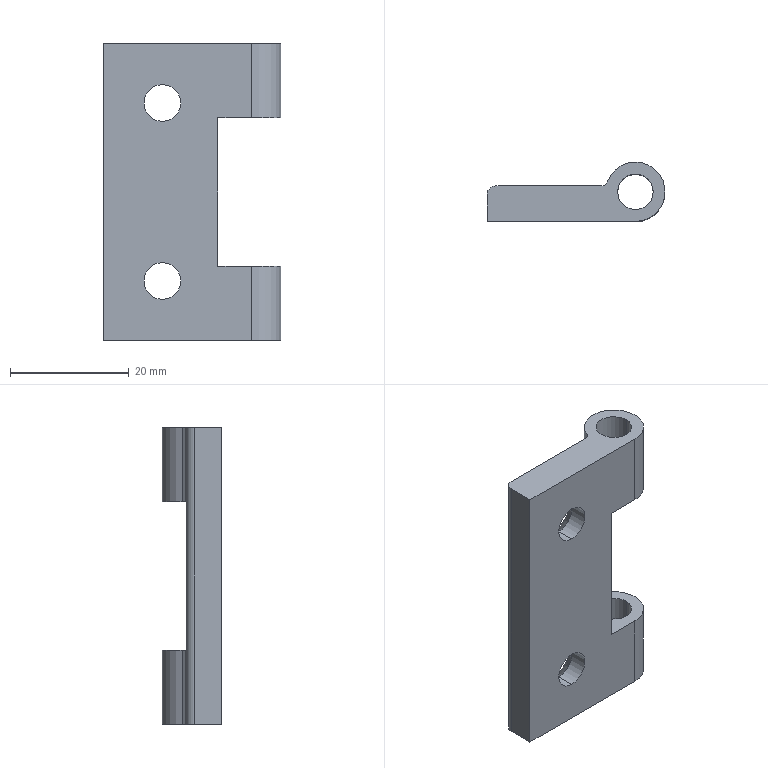Part | STEP file | 750038561 | 1 solid | 25 faces | box 30 x 10 x 50 mm | volume 6694 mm3 | cylinder 13 | plane 8 | cone 4 | commonest cylinder face diameters 6 x4 6.2 x4 2 x2 10 x2 3 x1
STEP:
#1=CARTESIAN_POINT('',(-15.,0.,18.1));
#2=VERTEX_POINT('',#1);
#3=CARTESIAN_POINT('',(-15.,0.,11.9));
#4=VERTEX_POINT('',#3);
#5=CARTESIAN_POINT('',(-15.,0.,15.));
#6=DIRECTION('',(0.,-1.,0.));
#7=DIRECTION('',(0.,0.,1.));
#8=AXIS2_PLACEMENT_3D('',#5,#6,#7);
#9=CIRCLE('',#8,3.1);
#10=EDGE_CURVE('',#2,#4,#9,.T.);
#11=ORIENTED_EDGE('',*,*,#10,.T.);
#12=CARTESIAN_POINT('',(-15.,3.1,11.9));
#13=VERTEX_POINT('',#12);
#14=CARTESIAN_POINT('',(-15.,-54994.,11.9));
#15=DIRECTION('',(0.,1.,0.));
#16=VECTOR('',#15,1000.);
#17=LINE('',#14,#16);
#18=EDGE_CURVE('',#4,#13,#17,.T.);
#19=ORIENTED_EDGE('',*,*,#18,.T.);
#20=CARTESIAN_POINT('',(-15.,3.1,18.1));
#21=VERTEX_POINT('',#20);
#22=CARTESIAN_POINT('',(-15.,3.1,15.));
#23=DIRECTION('',(0.,-1.,0.));
#24=DIRECTION('',(0.,0.,1.));
#25=AXIS2_PLACEMENT_3D('',#22,#23,#24);
#26=CIRCLE('',#25,3.1);
#27=EDGE_CURVE('',#21,#13,#26,.T.);
#28=ORIENTED_EDGE('',*,*,#27,.F.);
#29=CARTESIAN_POINT('',(-15.,-54994.,18.1));
#30=DIRECTION('',(0.,1.,0.));
#31=VECTOR('',#30,1000.);
#32=LINE('',#29,#31);
#33=EDGE_CURVE('',#2,#21,#32,.T.);
#34=ORIENTED_EDGE('',*,*,#33,.F.);
#35=EDGE_LOOP('',(#11,#19,#28,#34));
#36=FACE_OUTER_BOUND('',#35,.T.);
#37=CARTESIAN_POINT('',(-15.,-54994.,15.));
#38=DIRECTION('',(0.,1.,0.));
#39=DIRECTION('',(0.,0.,1.));
#40=AXIS2_PLACEMENT_3D('',#37,#38,#39);
#41=CYLINDRICAL_SURFACE('',#40,3.1);
#42=ADVANCED_FACE('',(#36),#41,.F.);
#43=CARTESIAN_POINT('',(-15.,0.,-11.9));
#44=VERTEX_POINT('',#43);
#45=CARTESIAN_POINT('',(-15.,0.,-18.1));
#46=VERTEX_POINT('',#45);
#47=CARTESIAN_POINT('',(-15.,0.,-15.));
#48=DIRECTION('',(0.,-1.,0.));
#49=DIRECTION('',(0.,0.,1.));
#50=AXIS2_PLACEMENT_3D('',#47,#48,#49);
#51=CIRCLE('',#50,3.1);
#52=EDGE_CURVE('',#44,#46,#51,.T.);
#53=ORIENTED_EDGE('',*,*,#52,.T.);
#54=CARTESIAN_POINT('',(-15.,3.1,-18.1));
#55=VERTEX_POINT('',#54);
#56=CARTESIAN_POINT('',(-15.,-54994.,-18.1));
#57=DIRECTION('',(0.,1.,0.));
#58=VECTOR('',#57,1000.);
#59=LINE('',#56,#58);
#60=EDGE_CURVE('',#46,#55,#59,.T.);
#61=ORIENTED_EDGE('',*,*,#60,.T.);
#62=CARTESIAN_POINT('',(-15.,3.1,-11.9));
#63=VERTEX_POINT('',#62);
#64=CARTESIAN_POINT('',(-15.,3.1,-15.));
#65=DIRECTION('',(0.,-1.,0.));
#66=DIRECTION('',(0.,0.,1.));
#67=AXIS2_PLACEMENT_3D('',#64,#65,#66);
#68=CIRCLE('',#67,3.1);
#69=EDGE_CURVE('',#63,#55,#68,.T.);
#70=ORIENTED_EDGE('',*,*,#69,.F.);
#71=CARTESIAN_POINT('',(-15.,-54994.,-11.9));
#72=DIRECTION('',(0.,1.,0.));
#73=VECTOR('',#72,1000.);
#74=LINE('',#71,#73);
#75=EDGE_CURVE('',#44,#63,#74,.T.);
#76=ORIENTED_EDGE('',*,*,#75,.F.);
#77=EDGE_LOOP('',(#53,#61,#70,#76));
#78=FACE_OUTER_BOUND('',#77,.T.);
#79=CARTESIAN_POINT('',(-15.,-54994.,-15.));
#80=DIRECTION('',(0.,1.,0.));
#81=DIRECTION('',(0.,0.,1.));
#82=AXIS2_PLACEMENT_3D('',#79,#80,#81);
#83=CYLINDRICAL_SURFACE('',#82,3.1);
#84=ADVANCED_FACE('',(#78),#83,.F.);
#85=CARTESIAN_POINT('',(3.,5.,25.));
#86=VERTEX_POINT('',#85);
#87=CARTESIAN_POINT('',(-3.,5.,25.));
#88=VERTEX_POINT('',#87);
#89=CARTESIAN_POINT('',(0.,5.,25.));
#90=DIRECTION('',(0.,0.,-1.));
#91=DIRECTION('',(-1.,0.,0.));
#92=AXIS2_PLACEMENT_3D('',#89,#90,#91);
#93=CIRCLE('',#92,3.);
#94=EDGE_CURVE('',#86,#88,#93,.T.);
#95=ORIENTED_EDGE('',*,*,#94,.F.);
#96=CARTESIAN_POINT('',(3.,5.,12.5));
#97=VERTEX_POINT('',#96);
#98=CARTESIAN_POINT('',(3.,5.,25.));
#99=DIRECTION('',(0.,0.,-1.));
#100=VECTOR('',#99,1000.);
#101=LINE('',#98,#100);
#102=EDGE_CURVE('',#86,#97,#101,.T.);
#103=ORIENTED_EDGE('',*,*,#102,.T.);
#104=CARTESIAN_POINT('',(-3.,5.,12.5));
#105=VERTEX_POINT('',#104);
#106=CARTESIAN_POINT('',(0.,5.,12.5));
#107=DIRECTION('',(0.,0.,1.));
#108=DIRECTION('',(-1.,0.,0.));
#109=AXIS2_PLACEMENT_3D('',#106,#107,#108);
#110=CIRCLE('',#109,3.);
#111=EDGE_CURVE('',#105,#97,#110,.T.);
#112=ORIENTED_EDGE('',*,*,#111,.F.);
#113=CARTESIAN_POINT('',(-3.,5.,25.));
#114=DIRECTION('',(0.,0.,-1.));
#115=VECTOR('',#114,1000.);
#116=LINE('',#113,#115);
#117=EDGE_CURVE('',#88,#105,#116,.T.);
#118=ORIENTED_EDGE('',*,*,#117,.F.);
#119=EDGE_LOOP('',(#95,#103,#112,#118));
#120=FACE_OUTER_BOUND('',#119,.T.);
#121=CARTESIAN_POINT('',(0.,5.,25.));
#122=DIRECTION('',(0.,0.,-1.));
#123=DIRECTION('',(-1.,0.,0.));
#124=AXIS2_PLACEMENT_3D('',#121,#122,#123);
#125=CYLINDRICAL_SURFACE('',#124,3.);
#126=ADVANCED_FACE('',(#120),#125,.F.);
#127=CARTESIAN_POINT('',(3.,5.,-12.5));
#128=VERTEX_POINT('',#127);
#129=CARTESIAN_POINT('',(-3.,5.,-12.5));
#130=VERTEX_POINT('',#129);
#131=CARTESIAN_POINT('',(0.,5.,-12.5));
#132=DIRECTION('',(0.,0.,-1.));
#133=DIRECTION('',(-1.,0.,0.));
#134=AXIS2_PLACEMENT_3D('',#131,#132,#133);
#135=CIRCLE('',#134,3.);
#136=EDGE_CURVE('',#128,#130,#135,.T.);
#137=ORIENTED_EDGE('',*,*,#136,.F.);
#138=CARTESIAN_POINT('',(3.,5.,-25.));
#139=VERTEX_POINT('',#138);
#140=CARTESIAN_POINT('',(3.,5.,25.));
#141=DIRECTION('',(0.,0.,-1.));
#142=VECTOR('',#141,1000.);
#143=LINE('',#140,#142);
#144=EDGE_CURVE('',#128,#139,#143,.T.);
#145=ORIENTED_EDGE('',*,*,#144,.T.);
#146=CARTESIAN_POINT('',(-3.,5.,-25.));
#147=VERTEX_POINT('',#146);
#148=CARTESIAN_POINT('',(0.,5.,-25.));
#149=DIRECTION('',(0.,0.,-1.));
#150=DIRECTION('',(-1.,0.,0.));
#151=AXIS2_PLACEMENT_3D('',#148,#149,#150);
#152=CIRCLE('',#151,3.);
#153=EDGE_CURVE('',#139,#147,#152,.T.);
#154=ORIENTED_EDGE('',*,*,#153,.T.);
#155=CARTESIAN_POINT('',(-3.,5.,25.));
#156=DIRECTION('',(0.,0.,-1.));
#157=VECTOR('',#156,1000.);
#158=LINE('',#155,#157);
#159=EDGE_CURVE('',#130,#147,#158,.T.);
#160=ORIENTED_EDGE('',*,*,#159,.F.);
#161=EDGE_LOOP('',(#137,#145,#154,#160));
#162=FACE_OUTER_BOUND('',#161,.T.);
#163=CARTESIAN_POINT('',(0.,5.,25.));
#164=DIRECTION('',(0.,0.,-1.));
#165=DIRECTION('',(-1.,0.,0.));
#166=AXIS2_PLACEMENT_3D('',#163,#164,#165);
#167=CYLINDRICAL_SURFACE('',#166,3.);
#168=ADVANCED_FACE('',(#162),#167,.F.);
#169=ORIENTED_EDGE('',*,*,#27,.T.);
#170=CARTESIAN_POINT('',(-15.,6.,9.));
#171=VERTEX_POINT('',#170);
#172=CARTESIAN_POINT('',(-15.,6.,9.));
#173=DIRECTION('',(0.,0.7071,-0.7071));
#174=VECTOR('',#173,1000.);
#175=LINE('',#172,#174);
#176=EDGE_CURVE('',#13,#171,#175,.T.);
#177=ORIENTED_EDGE('',*,*,#176,.T.);
#178=CARTESIAN_POINT('',(-15.,6.,21.));
#179=VERTEX_POINT('',#178);
#180=CARTESIAN_POINT('',(-15.,6.,15.));
#181=DIRECTION('',(0.,1.,0.));
#182=DIRECTION('',(0.,0.,1.));
#183=AXIS2_PLACEMENT_3D('',#180,#181,#182);
#184=CIRCLE('',#183,6.);
#185=EDGE_CURVE('',#171,#179,#184,.T.);
#186=ORIENTED_EDGE('',*,*,#185,.T.);
#187=CARTESIAN_POINT('',(-15.,6.,21.));
#188=DIRECTION('',(0.,0.7071,0.7071));
#189=VECTOR('',#188,1000.);
#190=LINE('',#187,#189);
#191=EDGE_CURVE('',#21,#179,#190,.T.);
#192=ORIENTED_EDGE('',*,*,#191,.F.);
#193=EDGE_LOOP('',(#169,#177,#186,#192));
#194=FACE_OUTER_BOUND('',#193,.T.);
#195=CARTESIAN_POINT('',(-15.,6.,15.));
#196=DIRECTION('',(0.,1.,0.));
#197=DIRECTION('',(0.,0.,1.));
#198=AXIS2_PLACEMENT_3D('',#195,#196,#197);
#199=CONICAL_SURFACE('',#198,6.,0.7854);
#200=ADVANCED_FACE('',(#194),#199,.F.);
#201=ORIENTED_EDGE('',*,*,#69,.T.);
#202=CARTESIAN_POINT('',(-15.,6.,-21.));
#203=VERTEX_POINT('',#202);
#204=CARTESIAN_POINT('',(-15.,6.,-21.));
#205=DIRECTION('',(0.,0.7071,-0.7071));
#206=VECTOR('',#205,1000.);
#207=LINE('',#204,#206);
#208=EDGE_CURVE('',#55,#203,#207,.T.);
#209=ORIENTED_EDGE('',*,*,#208,.T.);
#210=CARTESIAN_POINT('',(-15.,6.,-9.));
#211=VERTEX_POINT('',#210);
#212=CARTESIAN_POINT('',(-15.,6.,-15.));
#213=DIRECTION('',(0.,1.,0.));
#214=DIRECTION('',(0.,0.,1.));
#215=AXIS2_PLACEMENT_3D('',#212,#213,#214);
#216=CIRCLE('',#215,6.);
#217=EDGE_CURVE('',#203,#211,#216,.T.);
#218=ORIENTED_EDGE('',*,*,#217,.T.);
#219=CARTESIAN_POINT('',(-15.,6.,-9.));
#220=DIRECTION('',(0.,0.7071,0.7071));
#221=VECTOR('',#220,1000.);
#222=LINE('',#219,#221);
#223=EDGE_CURVE('',#63,#211,#222,.T.);
#224=ORIENTED_EDGE('',*,*,#223,.F.);
#225=EDGE_LOOP('',(#201,#209,#218,#224));
#226=FACE_OUTER_BOUND('',#225,.T.);
#227=CARTESIAN_POINT('',(-15.,6.,-15.));
#228=DIRECTION('',(0.,1.,0.));
#229=DIRECTION('',(0.,0.,1.));
#230=AXIS2_PLACEMENT_3D('',#227,#228,#229);
#231=CONICAL_SURFACE('',#230,6.,0.7854);
#232=ADVANCED_FACE('',(#226),#231,.F.);
#233=CARTESIAN_POINT('',(0.,0.,25.));
#234=VERTEX_POINT('',#233);
#235=CARTESIAN_POINT('',(0.,0.,12.5));
#236=VERTEX_POINT('',#235);
#237=CARTESIAN_POINT('',(0.,0.,25.));
#238=DIRECTION('',(0.,0.,-1.));
#239=VECTOR('',#238,1000.);
#240=LINE('',#237,#239);
#241=EDGE_CURVE('',#234,#236,#240,.T.);
#242=ORIENTED_EDGE('',*,*,#241,.F.);
#243=CARTESIAN_POINT('',(-25.,0.,25.));
#244=VERTEX_POINT('',#243);
#245=CARTESIAN_POINT('',(-25.,0.,25.));
#246=DIRECTION('',(1.,0.,0.));
#247=VECTOR('',#246,1000.);
#248=LINE('',#245,#247);
#249=EDGE_CURVE('',#244,#234,#248,.T.);
#250=ORIENTED_EDGE('',*,*,#249,.F.);
#251=CARTESIAN_POINT('',(-25.,0.,-25.));
#252=VERTEX_POINT('',#251);
#253=CARTESIAN_POINT('',(-25.,0.,25.));
#254=DIRECTION('',(0.,0.,1.));
#255=VECTOR('',#254,1000.);
#256=LINE('',#253,#255);
#257=EDGE_CURVE('',#252,#244,#256,.T.);
#258=ORIENTED_EDGE('',*,*,#257,.F.);
#259=CARTESIAN_POINT('',(0.,0.,-25.));
#260=VERTEX_POINT('',#259);
#261=CARTESIAN_POINT('',(-25.,0.,-25.));
#262=DIRECTION('',(-1.,0.,0.));
#263=VECTOR('',#262,1000.);
#264=LINE('',#261,#263);
#265=EDGE_CURVE('',#260,#252,#264,.T.);
#266=ORIENTED_EDGE('',*,*,#265,.F.);
#267=CARTESIAN_POINT('',(0.,0.,-12.5));
#268=VERTEX_POINT('',#267);
#269=CARTESIAN_POINT('',(0.,0.,25.));
#270=DIRECTION('',(0.,0.,-1.));
#271=VECTOR('',#270,1000.);
#272=LINE('',#269,#271);
#273=EDGE_CURVE('',#268,#260,#272,.T.);
#274=ORIENTED_EDGE('',*,*,#273,.F.);
#275=CARTESIAN_POINT('',(-5.657,0.,-12.5));
#276=VERTEX_POINT('',#275);
#277=CARTESIAN_POINT('',(-25.,0.,-12.5));
#278=DIRECTION('',(1.,0.,0.));
#279=VECTOR('',#278,1000.);
#280=LINE('',#277,#279);
#281=EDGE_CURVE('',#276,#268,#280,.T.);
#282=ORIENTED_EDGE('',*,*,#281,.F.);
#283=CARTESIAN_POINT('',(-5.657,0.,12.5));
#284=VERTEX_POINT('',#283);
#285=CARTESIAN_POINT('',(-5.657,0.,25.));
#286=DIRECTION('',(0.,0.,-1.));
#287=VECTOR('',#286,1000.);
#288=LINE('',#285,#287);
#289=EDGE_CURVE('',#284,#276,#288,.T.);
#290=ORIENTED_EDGE('',*,*,#289,.F.);
#291=CARTESIAN_POINT('',(-25.,0.,12.5));
#292=DIRECTION('',(-1.,0.,0.));
#293=VECTOR('',#292,1000.);
#294=LINE('',#291,#293);
#295=EDGE_CURVE('',#236,#284,#294,.T.);
#296=ORIENTED_EDGE('',*,*,#295,.F.);
#297=EDGE_LOOP('',(#242,#250,#258,#266,#274,#282,#290,#296));
#298=FACE_OUTER_BOUND('',#297,.T.);
#299=ORIENTED_EDGE('',*,*,#10,.F.);
#300=CARTESIAN_POINT('',(-15.,0.,15.));
#301=DIRECTION('',(0.,-1.,0.));
#302=DIRECTION('',(0.,0.,1.));
#303=AXIS2_PLACEMENT_3D('',#300,#301,#302);
#304=CIRCLE('',#303,3.1);
#305=EDGE_CURVE('',#4,#2,#304,.T.);
#306=ORIENTED_EDGE('',*,*,#305,.F.);
#307=EDGE_LOOP('',(#299,#306));
#308=FACE_BOUND('',#307,.T.);
#309=ORIENTED_EDGE('',*,*,#52,.F.);
#310=CARTESIAN_POINT('',(-15.,0.,-15.));
#311=DIRECTION('',(0.,-1.,0.));
#312=DIRECTION('',(0.,0.,1.));
#313=AXIS2_PLACEMENT_3D('',#310,#311,#312);
#314=CIRCLE('',#313,3.1);
#315=EDGE_CURVE('',#46,#44,#314,.T.);
#316=ORIENTED_EDGE('',*,*,#315,.F.);
#317=EDGE_LOOP('',(#309,#316));
#318=FACE_BOUND('',#317,.T.);
#319=CARTESIAN_POINT('',(-25.,0.,25.));
#320=DIRECTION('',(0.,1.,0.));
#321=DIRECTION('',(-1.,0.,0.));
#322=AXIS2_PLACEMENT_3D('',#319,#320,#321);
#323=PLANE('',#322);
#324=ADVANCED_FACE('',(#298,#308,#318),#323,.F.);
#325=CARTESIAN_POINT('',(-5.657,6.,12.5));
#326=VERTEX_POINT('',#325);
#327=CARTESIAN_POINT('',(-4.714,6.667,12.5));
#328=VERTEX_POINT('',#327);
#329=CARTESIAN_POINT('',(-5.657,7.,12.5));
#330=DIRECTION('',(0.,0.,1.));
#331=DIRECTION('',(-1.,0.,0.));
#332=AXIS2_PLACEMENT_3D('',#329,#330,#331);
#333=CIRCLE('',#332,1.);
#334=EDGE_CURVE('',#326,#328,#333,.T.);
#335=ORIENTED_EDGE('',*,*,#334,.T.);
#336=CARTESIAN_POINT('',(0.,5.,12.5));
#337=DIRECTION('',(0.,0.,-1.));
#338=DIRECTION('',(-1.,0.,0.));
#339=AXIS2_PLACEMENT_3D('',#336,#337,#338);
#340=CIRCLE('',#339,5.);
#341=EDGE_CURVE('',#328,#236,#340,.T.);
#342=ORIENTED_EDGE('',*,*,#341,.T.);
#343=ORIENTED_EDGE('',*,*,#295,.T.);
#344=CARTESIAN_POINT('',(-5.657,31.,12.5));
#345=DIRECTION('',(0.,1.,0.));
#346=VECTOR('',#345,1000.);
#347=LINE('',#344,#346);
#348=EDGE_CURVE('',#284,#326,#347,.T.);
#349=ORIENTED_EDGE('',*,*,#348,.T.);
#350=EDGE_LOOP('',(#335,#342,#343,#349));
#351=FACE_OUTER_BOUND('',#350,.T.);
#352=ORIENTED_EDGE('',*,*,#111,.T.);
#353=CARTESIAN_POINT('',(0.,5.,12.5));
#354=DIRECTION('',(0.,0.,1.));
#355=DIRECTION('',(-1.,0.,0.));
#356=AXIS2_PLACEMENT_3D('',#353,#354,#355);
#357=CIRCLE('',#356,3.);
#358=EDGE_CURVE('',#97,#105,#357,.T.);
#359=ORIENTED_EDGE('',*,*,#358,.T.);
#360=EDGE_LOOP('',(#352,#359));
#361=FACE_BOUND('',#360,.T.);
#362=CARTESIAN_POINT('',(-5.657,31.,12.5));
#363=DIRECTION('',(0.,0.,-1.));
#364=DIRECTION('',(-1.,0.,0.));
#365=AXIS2_PLACEMENT_3D('',#362,#363,#364);
#366=PLANE('',#365);
#367=ADVANCED_FACE('',(#351,#361),#366,.T.);
#368=CARTESIAN_POINT('',(-4.714,6.667,25.));
#369=VERTEX_POINT('',#368);
#370=CARTESIAN_POINT('',(0.,5.,25.));
#371=DIRECTION('',(0.,0.,-1.));
#372=DIRECTION('',(-1.,0.,0.));
#373=AXIS2_PLACEMENT_3D('',#370,#371,#372);
#374=CIRCLE('',#373,5.);
#375=EDGE_CURVE('',#369,#234,#374,.T.);
#376=ORIENTED_EDGE('',*,*,#375,.T.);
#377=ORIENTED_EDGE('',*,*,#241,.T.);
#378=ORIENTED_EDGE('',*,*,#341,.F.);
#379=CARTESIAN_POINT('',(-4.714,6.667,25.));
#380=DIRECTION('',(0.,0.,1.));
#381=VECTOR('',#380,1000.);
#382=LINE('',#379,#381);
#383=EDGE_CURVE('',#328,#369,#382,.T.);
#384=ORIENTED_EDGE('',*,*,#383,.T.);
#385=EDGE_LOOP('',(#376,#377,#378,#384));
#386=FACE_OUTER_BOUND('',#385,.T.);
#387=CARTESIAN_POINT('',(0.,5.,25.));
#388=DIRECTION('',(0.,0.,-1.));
#389=DIRECTION('',(-1.,0.,0.));
#390=AXIS2_PLACEMENT_3D('',#387,#388,#389);
#391=CYLINDRICAL_SURFACE('',#390,5.);
#392=ADVANCED_FACE('',(#386),#391,.T.);
#393=CARTESIAN_POINT('',(0.,5.,25.));
#394=DIRECTION('',(0.,0.,-1.));
#395=DIRECTION('',(-1.,0.,0.));
#396=AXIS2_PLACEMENT_3D('',#393,#394,#395);
#397=CIRCLE('',#396,3.);
#398=EDGE_CURVE('',#88,#86,#397,.T.);
#399=ORIENTED_EDGE('',*,*,#398,.T.);
#400=ORIENTED_EDGE('',*,*,#94,.T.);
#401=EDGE_LOOP('',(#399,#400));
#402=FACE_BOUND('',#401,.T.);
#403=CARTESIAN_POINT('',(-5.657,6.,25.));
#404=VERTEX_POINT('',#403);
#405=CARTESIAN_POINT('',(-23.5,6.,25.));
#406=VERTEX_POINT('',#405);
#407=CARTESIAN_POINT('',(0.,6.,25.));
#408=DIRECTION('',(-1.,0.,0.));
#409=VECTOR('',#408,1000.);
#410=LINE('',#407,#409);
#411=EDGE_CURVE('',#404,#406,#410,.T.);
#412=ORIENTED_EDGE('',*,*,#411,.T.);
#413=CARTESIAN_POINT('',(-25.,4.5,25.));
#414=VERTEX_POINT('',#413);
#415=CARTESIAN_POINT('',(-23.5,4.5,25.));
#416=DIRECTION('',(0.,0.,1.));
#417=DIRECTION('',(-1.,0.,0.));
#418=AXIS2_PLACEMENT_3D('',#415,#416,#417);
#419=CIRCLE('',#418,1.5);
#420=EDGE_CURVE('',#406,#414,#419,.T.);
#421=ORIENTED_EDGE('',*,*,#420,.T.);
#422=CARTESIAN_POINT('',(-25.,5.,25.));
#423=DIRECTION('',(0.,-1.,0.));
#424=VECTOR('',#423,1000.);
#425=LINE('',#422,#424);
#426=EDGE_CURVE('',#414,#244,#425,.T.);
#427=ORIENTED_EDGE('',*,*,#426,.T.);
#428=ORIENTED_EDGE('',*,*,#249,.T.);
#429=ORIENTED_EDGE('',*,*,#375,.F.);
#430=CARTESIAN_POINT('',(-5.657,7.,25.));
#431=DIRECTION('',(0.,0.,-1.));
#432=DIRECTION('',(-1.,0.,0.));
#433=AXIS2_PLACEMENT_3D('',#430,#431,#432);
#434=CIRCLE('',#433,1.);
#435=EDGE_CURVE('',#369,#404,#434,.T.);
#436=ORIENTED_EDGE('',*,*,#435,.T.);
#437=EDGE_LOOP('',(#412,#421,#427,#428,#429,#436));
#438=FACE_OUTER_BOUND('',#437,.T.);
#439=CARTESIAN_POINT('',(0.,5.,25.));
#440=DIRECTION('',(0.,0.,1.));
#441=DIRECTION('',(1.,0.,0.));
#442=AXIS2_PLACEMENT_3D('',#439,#440,#441);
#443=PLANE('',#442);
#444=ADVANCED_FACE('',(#402,#438),#443,.T.);
#445=ORIENTED_EDGE('',*,*,#257,.T.);
#446=ORIENTED_EDGE('',*,*,#426,.F.);
#447=CARTESIAN_POINT('',(-25.,4.5,-25.));
#448=VERTEX_POINT('',#447);
#449=CARTESIAN_POINT('',(-25.,4.5,25.));
#450=DIRECTION('',(0.,0.,1.));
#451=VECTOR('',#450,1000.);
#452=LINE('',#449,#451);
#453=EDGE_CURVE('',#448,#414,#452,.T.);
#454=ORIENTED_EDGE('',*,*,#453,.F.);
#455=CARTESIAN_POINT('',(-25.,4.5,-25.));
#456=DIRECTION('',(0.,1.,0.));
#457=VECTOR('',#456,1000.);
#458=LINE('',#455,#457);
#459=EDGE_CURVE('',#252,#448,#458,.T.);
#460=ORIENTED_EDGE('',*,*,#459,.F.);
#461=EDGE_LOOP('',(#445,#446,#454,#460));
#462=FACE_OUTER_BOUND('',#461,.T.);
#463=CARTESIAN_POINT('',(-25.,4.5,25.));
#464=DIRECTION('',(1.,0.,0.));
#465=DIRECTION('',(0.,0.,-1.));
#466=AXIS2_PLACEMENT_3D('',#463,#464,#465);
#467=PLANE('',#466);
#468=ADVANCED_FACE('',(#462),#467,.F.);
#469=CARTESIAN_POINT('',(0.,5.,-25.));
#470=DIRECTION('',(0.,0.,-1.));
#471=DIRECTION('',(-1.,0.,0.));
#472=AXIS2_PLACEMENT_3D('',#469,#470,#471);
#473=CIRCLE('',#472,3.);
#474=EDGE_CURVE('',#147,#139,#473,.T.);
#475=ORIENTED_EDGE('',*,*,#474,.F.);
#476=ORIENTED_EDGE('',*,*,#153,.F.);
#477=EDGE_LOOP('',(#475,#476));
#478=FACE_BOUND('',#477,.T.);
#479=CARTESIAN_POINT('',(-23.5,6.,-25.));
#480=VERTEX_POINT('',#479);
#481=CARTESIAN_POINT('',(-23.5,4.5,-25.));
#482=DIRECTION('',(0.,0.,1.));
#483=DIRECTION('',(-1.,0.,0.));
#484=AXIS2_PLACEMENT_3D('',#481,#482,#483);
#485=CIRCLE('',#484,1.5);
#486=EDGE_CURVE('',#480,#448,#485,.T.);
#487=ORIENTED_EDGE('',*,*,#486,.F.);
#488=CARTESIAN_POINT('',(-5.657,6.,-25.));
#489=VERTEX_POINT('',#488);
#490=CARTESIAN_POINT('',(0.,6.,-25.));
#491=DIRECTION('',(-1.,0.,0.));
#492=VECTOR('',#491,1000.);
#493=LINE('',#490,#492);
#494=EDGE_CURVE('',#489,#480,#493,.T.);
#495=ORIENTED_EDGE('',*,*,#494,.F.);
#496=CARTESIAN_POINT('',(-4.714,6.667,-25.));
#497=VERTEX_POINT('',#496);
#498=CARTESIAN_POINT('',(-5.657,7.,-25.));
#499=DIRECTION('',(0.,0.,1.));
#500=DIRECTION('',(-1.,0.,0.));
#501=AXIS2_PLACEMENT_3D('',#498,#499,#500);
#502=CIRCLE('',#501,1.);
#503=EDGE_CURVE('',#489,#497,#502,.T.);
#504=ORIENTED_EDGE('',*,*,#503,.T.);
#505=CARTESIAN_POINT('',(0.,5.,-25.));
#506=DIRECTION('',(0.,0.,1.));
#507=DIRECTION('',(-1.,0.,0.));
#508=AXIS2_PLACEMENT_3D('',#505,#506,#507);
#509=CIRCLE('',#508,5.);
#510=EDGE_CURVE('',#260,#497,#509,.T.);
#511=ORIENTED_EDGE('',*,*,#510,.F.);
#512=ORIENTED_EDGE('',*,*,#265,.T.);
#513=ORIENTED_EDGE('',*,*,#459,.T.);
#514=EDGE_LOOP('',(#487,#495,#504,#511,#512,#513));
#515=FACE_OUTER_BOUND('',#514,.T.);
#516=CARTESIAN_POINT('',(0.,5.,-25.));
#517=DIRECTION('',(0.,0.,1.));
#518=DIRECTION('',(1.,0.,0.));
#519=AXIS2_PLACEMENT_3D('',#516,#517,#518);
#520=PLANE('',#519);
#521=ADVANCED_FACE('',(#478,#515),#520,.F.);
#522=ORIENTED_EDGE('',*,*,#273,.T.);
#523=ORIENTED_EDGE('',*,*,#510,.T.);
#524=CARTESIAN_POINT('',(-4.714,6.667,-12.5));
#525=VERTEX_POINT('',#524);
#526=CARTESIAN_POINT('',(-4.714,6.667,25.));
#527=DIRECTION('',(0.,0.,1.));
#528=VECTOR('',#527,1000.);
#529=LINE('',#526,#528);
#530=EDGE_CURVE('',#497,#525,#529,.T.);
#531=ORIENTED_EDGE('',*,*,#530,.T.);
#532=CARTESIAN_POINT('',(0.,5.,-12.5));
#533=DIRECTION('',(0.,0.,-1.));
#534=DIRECTION('',(-1.,0.,0.));
#535=AXIS2_PLACEMENT_3D('',#532,#533,#534);
#536=CIRCLE('',#535,5.);
#537=EDGE_CURVE('',#525,#268,#536,.T.);
#538=ORIENTED_EDGE('',*,*,#537,.T.);
#539=EDGE_LOOP('',(#522,#523,#531,#538));
#540=FACE_OUTER_BOUND('',#539,.T.);
#541=CARTESIAN_POINT('',(0.,5.,25.));
#542=DIRECTION('',(0.,0.,-1.));
#543=DIRECTION('',(-1.,0.,0.));
#544=AXIS2_PLACEMENT_3D('',#541,#542,#543);
#545=CYLINDRICAL_SURFACE('',#544,5.);
#546=ADVANCED_FACE('',(#540),#545,.T.);
#547=CARTESIAN_POINT('',(-5.657,6.,-12.5));
#548=VERTEX_POINT('',#547);
#549=CARTESIAN_POINT('',(-5.657,7.,-12.5));
#550=DIRECTION('',(0.,0.,-1.));
#551=DIRECTION('',(-1.,0.,0.));
#552=AXIS2_PLACEMENT_3D('',#549,#550,#551);
#553=CIRCLE('',#552,1.);
#554=EDGE_CURVE('',#525,#548,#553,.T.);
#555=ORIENTED_EDGE('',*,*,#554,.T.);
#556=CARTESIAN_POINT('',(-5.657,31.,-12.5));
#557=DIRECTION('',(0.,-1.,0.));
#558=VECTOR('',#557,1000.);
#559=LINE('',#556,#558);
#560=EDGE_CURVE('',#548,#276,#559,.T.);
#561=ORIENTED_EDGE('',*,*,#560,.T.);
#562=ORIENTED_EDGE('',*,*,#281,.T.);
#563=ORIENTED_EDGE('',*,*,#537,.F.);
#564=EDGE_LOOP('',(#555,#561,#562,#563));
#565=FACE_OUTER_BOUND('',#564,.T.);
#566=CARTESIAN_POINT('',(0.,5.,-12.5));
#567=DIRECTION('',(0.,0.,-1.));
#568=DIRECTION('',(-1.,0.,0.));
#569=AXIS2_PLACEMENT_3D('',#566,#567,#568);
#570=CIRCLE('',#569,3.);
#571=EDGE_CURVE('',#130,#128,#570,.T.);
#572=ORIENTED_EDGE('',*,*,#571,.T.);
#573=ORIENTED_EDGE('',*,*,#136,.T.);
#574=EDGE_LOOP('',(#572,#573));
#575=FACE_BOUND('',#574,.T.);
#576=CARTESIAN_POINT('',(5.,31.,-12.5));
#577=DIRECTION('',(0.,0.,1.));
#578=DIRECTION('',(1.,0.,0.));
#579=AXIS2_PLACEMENT_3D('',#576,#577,#578);
#580=PLANE('',#579);
#581=ADVANCED_FACE('',(#565,#575),#580,.T.);
#582=CARTESIAN_POINT('',(-5.657,6.,-12.5));
#583=DIRECTION('',(0.,0.,1.));
#584=VECTOR('',#583,1000.);
#585=LINE('',#582,#584);
#586=EDGE_CURVE('',#548,#326,#585,.T.);
#587=ORIENTED_EDGE('',*,*,#586,.T.);
#588=ORIENTED_EDGE('',*,*,#348,.F.);
#589=ORIENTED_EDGE('',*,*,#289,.T.);
#590=ORIENTED_EDGE('',*,*,#560,.F.);
#591=EDGE_LOOP('',(#587,#588,#589,#590));
#592=FACE_OUTER_BOUND('',#591,.T.);
#593=CARTESIAN_POINT('',(-5.657,31.,-12.5));
#594=DIRECTION('',(1.,0.,0.));
#595=DIRECTION('',(0.,0.,-1.));
#596=AXIS2_PLACEMENT_3D('',#593,#594,#595);
#597=PLANE('',#596);
#598=ADVANCED_FACE('',(#592),#597,.T.);
#599=ORIENTED_EDGE('',*,*,#18,.F.);
#600=ORIENTED_EDGE('',*,*,#305,.T.);
#601=ORIENTED_EDGE('',*,*,#33,.T.);
#602=CARTESIAN_POINT('',(-15.,3.1,15.));
#603=DIRECTION('',(0.,-1.,0.));
#604=DIRECTION('',(0.,0.,1.));
#605=AXIS2_PLACEMENT_3D('',#602,#603,#604);
#606=CIRCLE('',#605,3.1);
#607=EDGE_CURVE('',#13,#21,#606,.T.);
#608=ORIENTED_EDGE('',*,*,#607,.F.);
#609=EDGE_LOOP('',(#599,#600,#601,#608));
#610=FACE_OUTER_BOUND('',#609,.T.);
#611=CARTESIAN_POINT('',(-15.,-54994.,15.));
#612=DIRECTION('',(0.,1.,0.));
#613=DIRECTION('',(0.,0.,1.));
#614=AXIS2_PLACEMENT_3D('',#611,#612,#613);
#615=CYLINDRICAL_SURFACE('',#614,3.1);
#616=ADVANCED_FACE('',(#610),#615,.F.);
#617=ORIENTED_EDGE('',*,*,#60,.F.);
#618=ORIENTED_EDGE('',*,*,#315,.T.);
#619=ORIENTED_EDGE('',*,*,#75,.T.);
#620=CARTESIAN_POINT('',(-15.,3.1,-15.));
#621=DIRECTION('',(0.,-1.,0.));
#622=DIRECTION('',(0.,0.,1.));
#623=AXIS2_PLACEMENT_3D('',#620,#621,#622);
#624=CIRCLE('',#623,3.1);
#625=EDGE_CURVE('',#55,#63,#624,.T.);
#626=ORIENTED_EDGE('',*,*,#625,.F.);
#627=EDGE_LOOP('',(#617,#618,#619,#626));
#628=FACE_OUTER_BOUND('',#627,.T.);
#629=CARTESIAN_POINT('',(-15.,-54994.,-15.));
#630=DIRECTION('',(0.,1.,0.));
#631=DIRECTION('',(0.,0.,1.));
#632=AXIS2_PLACEMENT_3D('',#629,#630,#631);
#633=CYLINDRICAL_SURFACE('',#632,3.1);
#634=ADVANCED_FACE('',(#628),#633,.F.);
#635=ORIENTED_EDGE('',*,*,#102,.F.);
#636=ORIENTED_EDGE('',*,*,#398,.F.);
#637=ORIENTED_EDGE('',*,*,#117,.T.);
#638=ORIENTED_EDGE('',*,*,#358,.F.);
#639=EDGE_LOOP('',(#635,#636,#637,#638));
#640=FACE_OUTER_BOUND('',#639,.T.);
#641=CARTESIAN_POINT('',(0.,5.,25.));
#642=DIRECTION('',(0.,0.,-1.));
#643=DIRECTION('',(-1.,0.,0.));
#644=AXIS2_PLACEMENT_3D('',#641,#642,#643);
#645=CYLINDRICAL_SURFACE('',#644,3.);
#646=ADVANCED_FACE('',(#640),#645,.F.);
#647=CARTESIAN_POINT('',(-5.657,6.,25.));
#648=DIRECTION('',(0.,0.,-1.));
#649=VECTOR('',#648,1000.);
#650=LINE('',#647,#649);
#651=EDGE_CURVE('',#404,#326,#650,.T.);
#652=ORIENTED_EDGE('',*,*,#651,.F.);
#653=ORIENTED_EDGE('',*,*,#435,.F.);
#654=ORIENTED_EDGE('',*,*,#383,.F.);
#655=ORIENTED_EDGE('',*,*,#334,.F.);
#656=EDGE_LOOP('',(#652,#653,#654,#655));
#657=FACE_OUTER_BOUND('',#656,.T.);
#658=CARTESIAN_POINT('',(-5.657,7.,25.));
#659=DIRECTION('',(0.,0.,-1.));
#660=DIRECTION('',(-1.,0.,0.));
#661=AXIS2_PLACEMENT_3D('',#658,#659,#660);
#662=CYLINDRICAL_SURFACE('',#661,1.);
#663=ADVANCED_FACE('',(#657),#662,.F.);
#664=ORIENTED_EDGE('',*,*,#420,.F.);
#665=CARTESIAN_POINT('',(-23.5,6.,25.));
#666=DIRECTION('',(0.,0.,-1.));
#667=VECTOR('',#666,1000.);
#668=LINE('',#665,#667);
#669=EDGE_CURVE('',#406,#480,#668,.T.);
#670=ORIENTED_EDGE('',*,*,#669,.T.);
#671=ORIENTED_EDGE('',*,*,#486,.T.);
#672=ORIENTED_EDGE('',*,*,#453,.T.);
#673=EDGE_LOOP('',(#664,#670,#671,#672));
#674=FACE_OUTER_BOUND('',#673,.T.);
#675=CARTESIAN_POINT('',(-23.5,4.5,25.));
#676=DIRECTION('',(0.,0.,-1.));
#677=DIRECTION('',(-1.,0.,0.));
#678=AXIS2_PLACEMENT_3D('',#675,#676,#677);
#679=CYLINDRICAL_SURFACE('',#678,1.5);
#680=ADVANCED_FACE('',(#674),#679,.T.);
#681=ORIENTED_EDGE('',*,*,#669,.F.);
#682=ORIENTED_EDGE('',*,*,#411,.F.);
#683=ORIENTED_EDGE('',*,*,#651,.T.);
#684=ORIENTED_EDGE('',*,*,#586,.F.);
#685=CARTESIAN_POINT('',(-5.657,6.,25.));
#686=DIRECTION('',(0.,0.,1.));
#687=VECTOR('',#686,1000.);
#688=LINE('',#685,#687);
#689=EDGE_CURVE('',#489,#548,#688,.T.);
#690=ORIENTED_EDGE('',*,*,#689,.F.);
#691=ORIENTED_EDGE('',*,*,#494,.T.);
#692=EDGE_LOOP('',(#681,#682,#683,#684,#690,#691));
#693=FACE_OUTER_BOUND('',#692,.T.);
#694=CARTESIAN_POINT('',(-15.,6.,-15.));
#695=DIRECTION('',(0.,1.,0.));
#696=DIRECTION('',(0.,0.,1.));
#697=AXIS2_PLACEMENT_3D('',#694,#695,#696);
#698=CIRCLE('',#697,6.);
#699=EDGE_CURVE('',#211,#203,#698,.T.);
#700=ORIENTED_EDGE('',*,*,#699,.F.);
#701=ORIENTED_EDGE('',*,*,#217,.F.);
#702=EDGE_LOOP('',(#700,#701));
#703=FACE_BOUND('',#702,.T.);
#704=CARTESIAN_POINT('',(-15.,6.,15.));
#705=DIRECTION('',(0.,1.,0.));
#706=DIRECTION('',(0.,0.,1.));
#707=AXIS2_PLACEMENT_3D('',#704,#705,#706);
#708=CIRCLE('',#707,6.);
#709=EDGE_CURVE('',#179,#171,#708,.T.);
#710=ORIENTED_EDGE('',*,*,#709,.F.);
#711=ORIENTED_EDGE('',*,*,#185,.F.);
#712=EDGE_LOOP('',(#710,#711));
#713=FACE_BOUND('',#712,.T.);
#714=CARTESIAN_POINT('',(-5.657,6.,25.));
#715=DIRECTION('',(0.,-1.,0.));
#716=DIRECTION('',(1.,0.,0.));
#717=AXIS2_PLACEMENT_3D('',#714,#715,#716);
#718=PLANE('',#717);
#719=ADVANCED_FACE('',(#693,#703,#713),#718,.F.);
#720=ORIENTED_EDGE('',*,*,#144,.F.);
#721=ORIENTED_EDGE('',*,*,#571,.F.);
#722=ORIENTED_EDGE('',*,*,#159,.T.);
#723=ORIENTED_EDGE('',*,*,#474,.T.);
#724=EDGE_LOOP('',(#720,#721,#722,#723));
#725=FACE_OUTER_BOUND('',#724,.T.);
#726=CARTESIAN_POINT('',(0.,5.,25.));
#727=DIRECTION('',(0.,0.,-1.));
#728=DIRECTION('',(-1.,0.,0.));
#729=AXIS2_PLACEMENT_3D('',#726,#727,#728);
#730=CYLINDRICAL_SURFACE('',#729,3.);
#731=ADVANCED_FACE('',(#725),#730,.F.);
#732=ORIENTED_EDGE('',*,*,#530,.F.);
#733=ORIENTED_EDGE('',*,*,#503,.F.);
#734=ORIENTED_EDGE('',*,*,#689,.T.);
#735=ORIENTED_EDGE('',*,*,#554,.F.);
#736=EDGE_LOOP('',(#732,#733,#734,#735));
#737=FACE_OUTER_BOUND('',#736,.T.);
#738=CARTESIAN_POINT('',(-5.657,7.,25.));
#739=DIRECTION('',(0.,0.,-1.));
#740=DIRECTION('',(-1.,0.,0.));
#741=AXIS2_PLACEMENT_3D('',#738,#739,#740);
#742=CYLINDRICAL_SURFACE('',#741,1.);
#743=ADVANCED_FACE('',(#737),#742,.F.);
#744=ORIENTED_EDGE('',*,*,#176,.F.);
#745=ORIENTED_EDGE('',*,*,#607,.T.);
#746=ORIENTED_EDGE('',*,*,#191,.T.);
#747=ORIENTED_EDGE('',*,*,#709,.T.);
#748=EDGE_LOOP('',(#744,#745,#746,#747));
#749=FACE_OUTER_BOUND('',#748,.T.);
#750=CARTESIAN_POINT('',(-15.,6.,15.));
#751=DIRECTION('',(0.,1.,0.));
#752=DIRECTION('',(0.,0.,1.));
#753=AXIS2_PLACEMENT_3D('',#750,#751,#752);
#754=CONICAL_SURFACE('',#753,6.,0.7854);
#755=ADVANCED_FACE('',(#749),#754,.F.);
#756=ORIENTED_EDGE('',*,*,#208,.F.);
#757=ORIENTED_EDGE('',*,*,#625,.T.);
#758=ORIENTED_EDGE('',*,*,#223,.T.);
#759=ORIENTED_EDGE('',*,*,#699,.T.);
#760=EDGE_LOOP('',(#756,#757,#758,#759));
#761=FACE_OUTER_BOUND('',#760,.T.);
#762=CARTESIAN_POINT('',(-15.,6.,-15.));
#763=DIRECTION('',(0.,1.,0.));
#764=DIRECTION('',(0.,0.,1.));
#765=AXIS2_PLACEMENT_3D('',#762,#763,#764);
#766=CONICAL_SURFACE('',#765,6.,0.7854);
#767=ADVANCED_FACE('',(#761),#766,.F.);
#768=CLOSED_SHELL('',(#42,#84,#126,#168,#200,#232,#324,#367,#392,#444,#468,#521,#546,#581,#598,#616,#634,#646,#663,#680,#719,#731,#743,#755,#767));
#769=MANIFOLD_SOLID_BREP('',#768);
#770=CARTESIAN_POINT('',(0.,0.,0.));
#771=DIRECTION('',(0.,0.,1.));
#772=DIRECTION('',(1.,0.,0.));
#773=AXIS2_PLACEMENT_3D('',#770,#771,#772);
#774=(LENGTH_UNIT()NAMED_UNIT(*)SI_UNIT(.MILLI.,.METRE.));
#775=UNCERTAINTY_MEASURE_WITH_UNIT(LENGTH_MEASURE(0.00001),#774,'','');
#776=(NAMED_UNIT(*)PLANE_ANGLE_UNIT()SI_UNIT($,.RADIAN.));
#777=(NAMED_UNIT(*)SI_UNIT($,.STERADIAN.)SOLID_ANGLE_UNIT());
#778=(GEOMETRIC_REPRESENTATION_CONTEXT(3)GLOBAL_UNCERTAINTY_ASSIGNED_CONTEXT((#775))GLOBAL_UNIT_ASSIGNED_CONTEXT((#774,#776,#777))REPRESENTATION_CONTEXT('',''));
#779=ADVANCED_BREP_SHAPE_REPRESENTATION('',(#769,#773),#778);